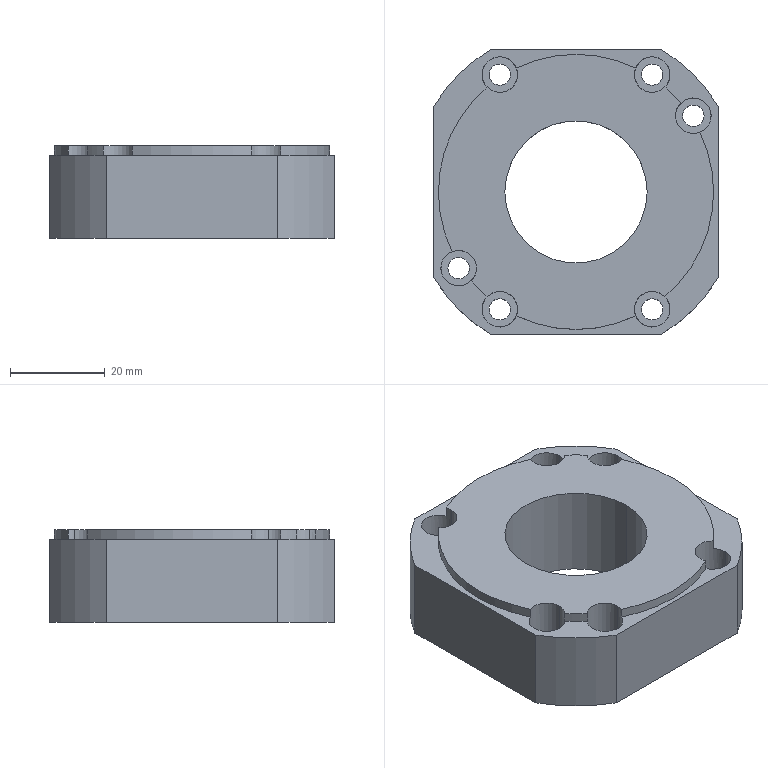Part | STEP file | _X2_8f9351657aef58f34f53_X0_MABR060.STEP_3.STEP_1.STEP_2.STEP.STEP | 1 solid | 50 faces | box 60 x 60 x 19.5 mm | volume 47406 mm3 | cylinder 37 | plane 13 | commonest cylinder face diameters 4.5 x12 7.5 x12 58 x7 70 x4 30 x2